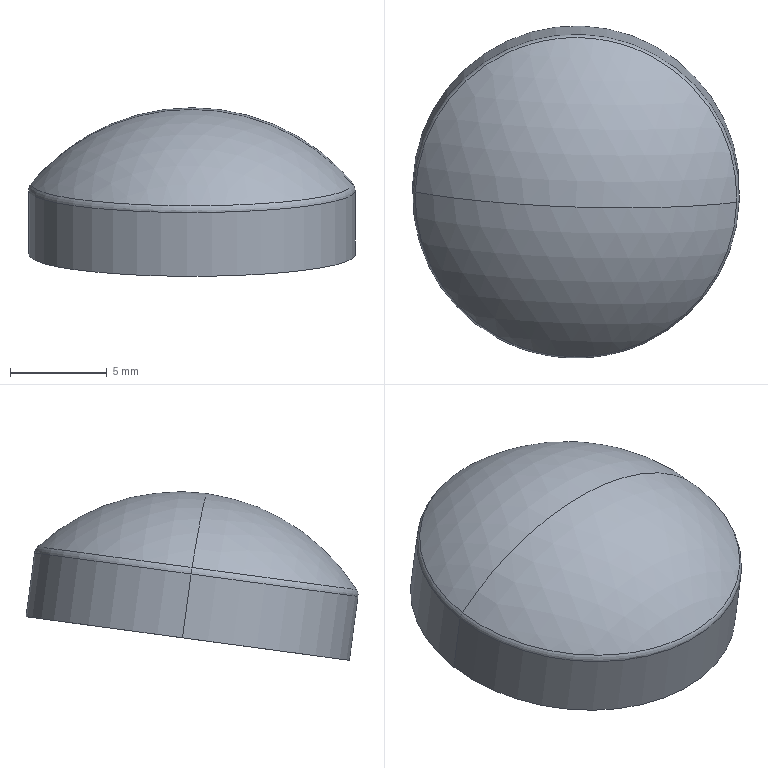Part | SolidWorks | features SplitBody 1 | 1 solid | 11 faces | box 16.896 x 17.194 x 8.727 mm | volume 214.231 mm3 | sphere 4 | cylinder 4 | torus 2 | plane 1 | commonest cylinder face diameters 15.84 x2 16.896 x2
STEP:
#1=CARTESIAN_POINT('',(552.494,359.862,-308.046));
#2=VERTEX_POINT('',#1);
#3=CARTESIAN_POINT('',(535.851,360.392,-307.975));
#4=VERTEX_POINT('',#3);
#5=CARTESIAN_POINT('',(544.173,360.127,-308.011));
#6=DIRECTION('',(0.,-0.1337,0.991));
#7=DIRECTION('',(0.9995,-0.03181,-0.00429));
#8=AXIS2_PLACEMENT_3D('',#5,#6,#7);
#9=CIRCLE('',#8,8.326);
#10=EDGE_CURVE('',#2,#4,#9,.T.);
#11=ORIENTED_EDGE('',*,*,#10,.T.);
#12=CARTESIAN_POINT('',(544.173,359.606,-304.147));
#13=VERTEX_POINT('',#12);
#14=CARTESIAN_POINT('',(544.173,361.055,-314.889));
#15=DIRECTION('',(0.0321,0.9905,0.1336));
#16=DIRECTION('',(0.,-0.1337,0.991));
#17=AXIS2_PLACEMENT_3D('',#14,#15,#16);
#18=CIRCLE('',#17,10.839);
#19=EDGE_CURVE('',#4,#13,#18,.T.);
#20=ORIENTED_EDGE('',*,*,#19,.T.);
#21=CARTESIAN_POINT('',(544.173,361.055,-314.889));
#22=DIRECTION('',(-0.0321,-0.9905,-0.1336));
#23=DIRECTION('',(0.,0.1337,-0.991));
#24=AXIS2_PLACEMENT_3D('',#21,#22,#23);
#25=CIRCLE('',#24,10.839);
#26=EDGE_CURVE('',#2,#13,#25,.T.);
#27=ORIENTED_EDGE('',*,*,#26,.F.);
#28=EDGE_LOOP('',(#11,#20,#27));
#29=FACE_OUTER_BOUND('',#28,.T.);
#30=CARTESIAN_POINT('',(544.173,361.055,-314.889));
#31=DIRECTION('',(0.0321,0.9905,0.1336));
#32=DIRECTION('',(0.9995,-0.03181,-0.00429));
#33=AXIS2_PLACEMENT_3D('',#30,#31,#32);
#34=SPHERICAL_SURFACE('',#33,10.839);
#35=ADVANCED_FACE('',(#29),#34,.T.);
#36=CARTESIAN_POINT('',(536.257,360.399,-308.125));
#37=VERTEX_POINT('',#36);
#38=CARTESIAN_POINT('',(552.088,359.895,-308.193));
#39=VERTEX_POINT('',#38);
#40=CARTESIAN_POINT('',(544.173,360.147,-308.159));
#41=DIRECTION('',(0.,0.1337,-0.991));
#42=DIRECTION('',(0.9995,-0.03181,-0.00429));
#43=AXIS2_PLACEMENT_3D('',#40,#41,#42);
#44=CIRCLE('',#43,7.92);
#45=EDGE_CURVE('',#37,#39,#44,.T.);
#46=ORIENTED_EDGE('',*,*,#45,.T.);
#47=CARTESIAN_POINT('',(544.173,359.676,-304.67));
#48=VERTEX_POINT('',#47);
#49=CARTESIAN_POINT('',(544.173,361.103,-315.245));
#50=DIRECTION('',(-0.0321,-0.9905,-0.1336));
#51=DIRECTION('',(0.,0.1337,-0.991));
#52=AXIS2_PLACEMENT_3D('',#49,#50,#51);
#53=CIRCLE('',#52,10.67);
#54=EDGE_CURVE('',#39,#48,#53,.T.);
#55=ORIENTED_EDGE('',*,*,#54,.T.);
#56=CARTESIAN_POINT('',(544.173,361.103,-315.245));
#57=DIRECTION('',(0.0321,0.9905,0.1336));
#58=DIRECTION('',(0.,-0.1337,0.991));
#59=AXIS2_PLACEMENT_3D('',#56,#57,#58);
#60=CIRCLE('',#59,10.67);
#61=EDGE_CURVE('',#37,#48,#60,.T.);
#62=ORIENTED_EDGE('',*,*,#61,.F.);
#63=EDGE_LOOP('',(#46,#55,#62));
#64=FACE_OUTER_BOUND('',#63,.T.);
#65=CARTESIAN_POINT('',(544.173,361.103,-315.245));
#66=DIRECTION('',(-0.0321,-0.9905,-0.1336));
#67=DIRECTION('',(-0.9995,0.03181,0.00429));
#68=AXIS2_PLACEMENT_3D('',#65,#66,#67);
#69=SPHERICAL_SURFACE('',#68,10.67);
#70=ADVANCED_FACE('',(#64),#69,.F.);
#71=CARTESIAN_POINT('',(536.257,360.869,-311.613));
#72=VERTEX_POINT('',#71);
#73=CARTESIAN_POINT('',(552.088,360.366,-311.681));
#74=VERTEX_POINT('',#73);
#75=CARTESIAN_POINT('',(544.173,360.617,-311.647));
#76=DIRECTION('',(0.,0.1337,-0.991));
#77=DIRECTION('',(0.9995,-0.03181,-0.00429));
#78=AXIS2_PLACEMENT_3D('',#75,#76,#77);
#79=CIRCLE('',#78,7.92);
#80=EDGE_CURVE('',#72,#74,#79,.T.);
#81=ORIENTED_EDGE('',*,*,#80,.T.);
#82=CARTESIAN_POINT('',(552.088,360.366,-311.681));
#83=DIRECTION('',(0.,-0.1337,0.991));
#84=VECTOR('',#83,1000.);
#85=LINE('',#82,#84);
#86=EDGE_CURVE('',#74,#39,#85,.T.);
#87=ORIENTED_EDGE('',*,*,#86,.T.);
#88=ORIENTED_EDGE('',*,*,#45,.F.);
#89=CARTESIAN_POINT('',(536.257,360.869,-311.613));
#90=DIRECTION('',(0.,-0.1337,0.991));
#91=VECTOR('',#90,1000.);
#92=LINE('',#89,#91);
#93=EDGE_CURVE('',#72,#37,#92,.T.);
#94=ORIENTED_EDGE('',*,*,#93,.F.);
#95=EDGE_LOOP('',(#81,#87,#88,#94));
#96=FACE_OUTER_BOUND('',#95,.T.);
#97=CARTESIAN_POINT('',(544.173,360.617,-311.647));
#98=DIRECTION('',(0.,-0.1337,0.991));
#99=DIRECTION('',(-0.9995,0.03181,0.00429));
#100=AXIS2_PLACEMENT_3D('',#97,#98,#99);
#101=CYLINDRICAL_SURFACE('',#100,7.92);
#102=ADVANCED_FACE('',(#96),#101,.F.);
#103=CARTESIAN_POINT('',(552.616,360.349,-311.683));
#104=VERTEX_POINT('',#103);
#105=CARTESIAN_POINT('',(535.729,360.886,-311.611));
#106=VERTEX_POINT('',#105);
#107=CARTESIAN_POINT('',(544.173,360.617,-311.647));
#108=DIRECTION('',(0.,0.1337,-0.991));
#109=DIRECTION('',(-0.0321,-0.9905,-0.1336));
#110=AXIS2_PLACEMENT_3D('',#107,#108,#109);
#111=CIRCLE('',#110,8.448);
#112=EDGE_CURVE('',#104,#106,#111,.T.);
#113=ORIENTED_EDGE('',*,*,#112,.F.);
#114=CARTESIAN_POINT('',(552.616,359.903,-308.382));
#115=VERTEX_POINT('',#114);
#116=CARTESIAN_POINT('',(552.616,360.349,-311.683));
#117=DIRECTION('',(0.,-0.1337,0.991));
#118=VECTOR('',#117,1000.);
#119=LINE('',#116,#118);
#120=EDGE_CURVE('',#104,#115,#119,.T.);
#121=ORIENTED_EDGE('',*,*,#120,.T.);
#122=CARTESIAN_POINT('',(535.729,360.441,-308.309));
#123=VERTEX_POINT('',#122);
#124=CARTESIAN_POINT('',(544.173,360.172,-308.346));
#125=DIRECTION('',(0.,0.1337,-0.991));
#126=DIRECTION('',(0.9995,-0.03181,-0.00429));
#127=AXIS2_PLACEMENT_3D('',#124,#125,#126);
#128=CIRCLE('',#127,8.448);
#129=EDGE_CURVE('',#115,#123,#128,.T.);
#130=ORIENTED_EDGE('',*,*,#129,.T.);
#131=CARTESIAN_POINT('',(535.729,360.886,-311.611));
#132=DIRECTION('',(0.,-0.1337,0.991));
#133=VECTOR('',#132,1000.);
#134=LINE('',#131,#133);
#135=EDGE_CURVE('',#106,#123,#134,.T.);
#136=ORIENTED_EDGE('',*,*,#135,.F.);
#137=EDGE_LOOP('',(#113,#121,#130,#136));
#138=FACE_OUTER_BOUND('',#137,.T.);
#139=CARTESIAN_POINT('',(544.173,360.617,-311.647));
#140=DIRECTION('',(0.,-0.1337,0.991));
#141=DIRECTION('',(-0.9995,0.03181,0.00429));
#142=AXIS2_PLACEMENT_3D('',#139,#140,#141);
#143=CYLINDRICAL_SURFACE('',#142,8.448);
#144=ADVANCED_FACE('',(#138),#143,.T.);
#145=CARTESIAN_POINT('',(544.173,360.127,-308.011));
#146=DIRECTION('',(0.,-0.1337,0.991));
#147=DIRECTION('',(0.9995,-0.03181,-0.00429));
#148=AXIS2_PLACEMENT_3D('',#145,#146,#147);
#149=CIRCLE('',#148,8.326);
#150=EDGE_CURVE('',#4,#2,#149,.T.);
#151=ORIENTED_EDGE('',*,*,#150,.F.);
#152=CARTESIAN_POINT('',(536.257,360.424,-308.312));
#153=DIRECTION('',(-0.0321,-0.9905,-0.1336));
#154=DIRECTION('',(0.,0.1337,-0.991));
#155=AXIS2_PLACEMENT_3D('',#152,#153,#154);
#156=CIRCLE('',#155,0.528);
#157=EDGE_CURVE('',#4,#123,#156,.T.);
#158=ORIENTED_EDGE('',*,*,#157,.T.);
#159=ORIENTED_EDGE('',*,*,#129,.F.);
#160=CARTESIAN_POINT('',(552.088,359.92,-308.38));
#161=DIRECTION('',(0.0321,0.9905,0.1336));
#162=DIRECTION('',(0.,-0.1337,0.991));
#163=AXIS2_PLACEMENT_3D('',#160,#161,#162);
#164=CIRCLE('',#163,0.528);
#165=EDGE_CURVE('',#2,#115,#164,.T.);
#166=ORIENTED_EDGE('',*,*,#165,.F.);
#167=EDGE_LOOP('',(#151,#158,#159,#166));
#168=FACE_OUTER_BOUND('',#167,.T.);
#169=CARTESIAN_POINT('',(544.173,360.172,-308.346));
#170=DIRECTION('',(0.,0.1337,-0.991));
#171=DIRECTION('',(0.9995,-0.03181,-0.00429));
#172=AXIS2_PLACEMENT_3D('',#169,#170,#171);
#173=TOROIDAL_SURFACE('',#172,7.92,0.528);
#174=ADVANCED_FACE('',(#168),#173,.T.);
#175=ORIENTED_EDGE('',*,*,#157,.F.);
#176=ORIENTED_EDGE('',*,*,#10,.F.);
#177=ORIENTED_EDGE('',*,*,#165,.T.);
#178=CARTESIAN_POINT('',(544.173,360.172,-308.346));
#179=DIRECTION('',(0.,0.1337,-0.991));
#180=DIRECTION('',(0.9995,-0.03181,-0.00429));
#181=AXIS2_PLACEMENT_3D('',#178,#179,#180);
#182=CIRCLE('',#181,8.448);
#183=EDGE_CURVE('',#123,#115,#182,.T.);
#184=ORIENTED_EDGE('',*,*,#183,.F.);
#185=EDGE_LOOP('',(#175,#176,#177,#184));
#186=FACE_OUTER_BOUND('',#185,.T.);
#187=CARTESIAN_POINT('',(544.173,360.172,-308.346));
#188=DIRECTION('',(0.,0.1337,-0.991));
#189=DIRECTION('',(0.9995,-0.03181,-0.00429));
#190=AXIS2_PLACEMENT_3D('',#187,#188,#189);
#191=TOROIDAL_SURFACE('',#190,7.92,0.528);
#192=ADVANCED_FACE('',(#186),#191,.T.);
#193=CARTESIAN_POINT('',(544.173,360.617,-311.647));
#194=DIRECTION('',(0.,0.1337,-0.991));
#195=DIRECTION('',(-0.0321,-0.9905,-0.1336));
#196=AXIS2_PLACEMENT_3D('',#193,#194,#195);
#197=CIRCLE('',#196,8.448);
#198=EDGE_CURVE('',#106,#104,#197,.T.);
#199=ORIENTED_EDGE('',*,*,#198,.T.);
#200=ORIENTED_EDGE('',*,*,#112,.T.);
#201=EDGE_LOOP('',(#199,#200));
#202=FACE_OUTER_BOUND('',#201,.T.);
#203=ORIENTED_EDGE('',*,*,#80,.F.);
#204=CARTESIAN_POINT('',(544.173,360.617,-311.647));
#205=DIRECTION('',(0.,0.1337,-0.991));
#206=DIRECTION('',(0.9995,-0.03181,-0.00429));
#207=AXIS2_PLACEMENT_3D('',#204,#205,#206);
#208=CIRCLE('',#207,7.92);
#209=EDGE_CURVE('',#74,#72,#208,.T.);
#210=ORIENTED_EDGE('',*,*,#209,.F.);
#211=EDGE_LOOP('',(#203,#210));
#212=FACE_BOUND('',#211,.T.);
#213=CARTESIAN_POINT('',(544.173,360.617,-311.647));
#214=DIRECTION('',(0.,0.1337,-0.991));
#215=DIRECTION('',(0.9995,-0.03181,-0.00429));
#216=AXIS2_PLACEMENT_3D('',#213,#214,#215);
#217=PLANE('',#216);
#218=ADVANCED_FACE('',(#202,#212),#217,.T.);
#219=ORIENTED_EDGE('',*,*,#120,.F.);
#220=ORIENTED_EDGE('',*,*,#198,.F.);
#221=ORIENTED_EDGE('',*,*,#135,.T.);
#222=ORIENTED_EDGE('',*,*,#183,.T.);
#223=EDGE_LOOP('',(#219,#220,#221,#222));
#224=FACE_OUTER_BOUND('',#223,.T.);
#225=CARTESIAN_POINT('',(544.173,360.617,-311.647));
#226=DIRECTION('',(0.,-0.1337,0.991));
#227=DIRECTION('',(-0.9995,0.03181,0.00429));
#228=AXIS2_PLACEMENT_3D('',#225,#226,#227);
#229=CYLINDRICAL_SURFACE('',#228,8.448);
#230=ADVANCED_FACE('',(#224),#229,.T.);
#231=ORIENTED_EDGE('',*,*,#86,.F.);
#232=ORIENTED_EDGE('',*,*,#209,.T.);
#233=ORIENTED_EDGE('',*,*,#93,.T.);
#234=CARTESIAN_POINT('',(544.173,360.147,-308.159));
#235=DIRECTION('',(0.,0.1337,-0.991));
#236=DIRECTION('',(0.9995,-0.03181,-0.00429));
#237=AXIS2_PLACEMENT_3D('',#234,#235,#236);
#238=CIRCLE('',#237,7.92);
#239=EDGE_CURVE('',#39,#37,#238,.T.);
#240=ORIENTED_EDGE('',*,*,#239,.F.);
#241=EDGE_LOOP('',(#231,#232,#233,#240));
#242=FACE_OUTER_BOUND('',#241,.T.);
#243=CARTESIAN_POINT('',(544.173,360.617,-311.647));
#244=DIRECTION('',(0.,-0.1337,0.991));
#245=DIRECTION('',(-0.9995,0.03181,0.00429));
#246=AXIS2_PLACEMENT_3D('',#243,#244,#245);
#247=CYLINDRICAL_SURFACE('',#246,7.92);
#248=ADVANCED_FACE('',(#242),#247,.F.);
#249=ORIENTED_EDGE('',*,*,#54,.F.);
#250=ORIENTED_EDGE('',*,*,#239,.T.);
#251=ORIENTED_EDGE('',*,*,#61,.T.);
#252=EDGE_LOOP('',(#249,#250,#251));
#253=FACE_OUTER_BOUND('',#252,.T.);
#254=CARTESIAN_POINT('',(544.173,361.103,-315.245));
#255=DIRECTION('',(-0.0321,-0.9905,-0.1336));
#256=DIRECTION('',(-0.9995,0.03181,0.00429));
#257=AXIS2_PLACEMENT_3D('',#254,#255,#256);
#258=SPHERICAL_SURFACE('',#257,10.67);
#259=ADVANCED_FACE('',(#253),#258,.F.);
#260=ORIENTED_EDGE('',*,*,#19,.F.);
#261=ORIENTED_EDGE('',*,*,#150,.T.);
#262=ORIENTED_EDGE('',*,*,#26,.T.);
#263=EDGE_LOOP('',(#260,#261,#262));
#264=FACE_OUTER_BOUND('',#263,.T.);
#265=CARTESIAN_POINT('',(544.173,361.055,-314.889));
#266=DIRECTION('',(0.0321,0.9905,0.1336));
#267=DIRECTION('',(0.9995,-0.03181,-0.00429));
#268=AXIS2_PLACEMENT_3D('',#265,#266,#267);
#269=SPHERICAL_SURFACE('',#268,10.839);
#270=ADVANCED_FACE('',(#264),#269,.T.);
#271=CLOSED_SHELL('',(#35,#70,#102,#144,#174,#192,#218,#230,#248,#259,#270));
#272=MANIFOLD_SOLID_BREP('',#271);
#273=CARTESIAN_POINT('',(0.,0.,0.));
#274=DIRECTION('',(0.,0.,1.));
#275=DIRECTION('',(1.,0.,0.));
#276=AXIS2_PLACEMENT_3D('',#273,#274,#275);
#277=(LENGTH_UNIT()NAMED_UNIT(*)SI_UNIT(.MILLI.,.METRE.));
#278=UNCERTAINTY_MEASURE_WITH_UNIT(LENGTH_MEASURE(0.00001),#277,'','');
#279=(NAMED_UNIT(*)PLANE_ANGLE_UNIT()SI_UNIT($,.RADIAN.));
#280=(NAMED_UNIT(*)SI_UNIT($,.STERADIAN.)SOLID_ANGLE_UNIT());
#281=(GEOMETRIC_REPRESENTATION_CONTEXT(3)GLOBAL_UNCERTAINTY_ASSIGNED_CONTEXT((#278))GLOBAL_UNIT_ASSIGNED_CONTEXT((#277,#279,#280))REPRESENTATION_CONTEXT('',''));
#282=ADVANCED_BREP_SHAPE_REPRESENTATION('',(#272,#276),#281);